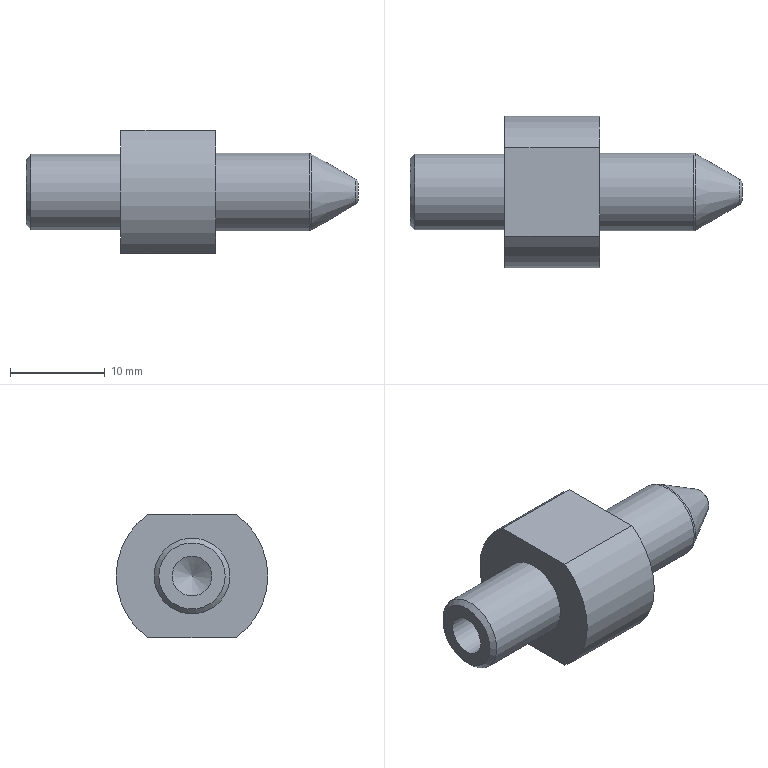Part | NX | features BREP 1 | 1 solid | 16 faces | box 35.023 x 16 x 13 mm | volume 2792 mm3 | plane 6 | cylinder 5 | cone 3 | torus 2 | commonest cylinder face diameters 16 x2 4.2 x1 8 x1 8.2 x1
STEP:
#1=CARTESIAN_POINT('',(2.489,-4.664,-6.5));
#2=VERTEX_POINT('',#1);
#3=CARTESIAN_POINT('',(2.489,-4.664,6.5));
#4=VERTEX_POINT('',#3);
#5=CARTESIAN_POINT('',(2.489,0.,0.));
#6=DIRECTION('',(-1.,0.,0.));
#7=DIRECTION('',(0.,-1.,0.));
#8=AXIS2_PLACEMENT_3D('',#5,#6,#7);
#9=CIRCLE('',#8,8.);
#10=EDGE_CURVE('',#2,#4,#9,.T.);
#11=ORIENTED_EDGE('',*,*,#10,.T.);
#12=CARTESIAN_POINT('',(-7.511,-4.664,6.5));
#13=VERTEX_POINT('',#12);
#14=CARTESIAN_POINT('',(-17.511,-4.664,6.5));
#15=DIRECTION('',(-1.,0.,0.));
#16=VECTOR('',#15,1000.);
#17=LINE('',#14,#16);
#18=EDGE_CURVE('',#4,#13,#17,.T.);
#19=ORIENTED_EDGE('',*,*,#18,.T.);
#20=CARTESIAN_POINT('',(-7.511,-4.664,-6.5));
#21=VERTEX_POINT('',#20);
#22=CARTESIAN_POINT('',(-7.511,0.,0.));
#23=DIRECTION('',(-1.,0.,0.));
#24=DIRECTION('',(0.,-1.,0.));
#25=AXIS2_PLACEMENT_3D('',#22,#23,#24);
#26=CIRCLE('',#25,8.);
#27=EDGE_CURVE('',#21,#13,#26,.T.);
#28=ORIENTED_EDGE('',*,*,#27,.F.);
#29=CARTESIAN_POINT('',(-17.511,-4.664,-6.5));
#30=DIRECTION('',(1.,0.,0.));
#31=VECTOR('',#30,1000.);
#32=LINE('',#29,#31);
#33=EDGE_CURVE('',#21,#2,#32,.T.);
#34=ORIENTED_EDGE('',*,*,#33,.T.);
#35=EDGE_LOOP('',(#11,#19,#28,#34));
#36=FACE_BOUND('',#35,.T.);
#37=CARTESIAN_POINT('',(-17.511,0.,0.));
#38=DIRECTION('',(-1.,0.,0.));
#39=DIRECTION('',(0.,1.,0.));
#40=AXIS2_PLACEMENT_3D('',#37,#38,#39);
#41=CYLINDRICAL_SURFACE('',#40,8.);
#42=ADVANCED_FACE('',(#36),#41,.T.);
#43=CARTESIAN_POINT('',(-17.511,3.5,0.));
#44=VERTEX_POINT('',#43);
#45=CARTESIAN_POINT('',(-17.511,0.,0.));
#46=DIRECTION('',(-1.,0.,0.));
#47=DIRECTION('',(0.,1.,0.));
#48=AXIS2_PLACEMENT_3D('',#45,#46,#47);
#49=CIRCLE('',#48,3.5);
#50=EDGE_CURVE('',#44,#44,#49,.T.);
#51=ORIENTED_EDGE('',*,*,#50,.T.);
#52=EDGE_LOOP('',(#51));
#53=FACE_BOUND('',#52,.T.);
#54=CARTESIAN_POINT('',(-17.511,0.,2.1));
#55=VERTEX_POINT('',#54);
#56=CARTESIAN_POINT('',(-17.511,0.,0.));
#57=DIRECTION('',(-1.,0.,0.));
#58=DIRECTION('',(0.,0.,1.));
#59=AXIS2_PLACEMENT_3D('',#56,#57,#58);
#60=CIRCLE('',#59,2.1);
#61=EDGE_CURVE('',#55,#55,#60,.T.);
#62=ORIENTED_EDGE('',*,*,#61,.F.);
#63=EDGE_LOOP('',(#62));
#64=FACE_BOUND('',#63,.T.);
#65=CARTESIAN_POINT('',(-17.511,4.,0.));
#66=DIRECTION('',(1.,0.,0.));
#67=DIRECTION('',(0.,-1.,0.));
#68=AXIS2_PLACEMENT_3D('',#65,#66,#67);
#69=PLANE('',#68);
#70=ADVANCED_FACE('',(#53,#64),#69,.F.);
#71=CARTESIAN_POINT('',(17.511,-0.9113,0.));
#72=VERTEX_POINT('',#71);
#73=CARTESIAN_POINT('',(17.511,0.,0.));
#74=DIRECTION('',(1.,0.,0.));
#75=DIRECTION('',(0.,-1.,0.));
#76=AXIS2_PLACEMENT_3D('',#73,#74,#75);
#77=CIRCLE('',#76,0.9113);
#78=EDGE_CURVE('',#72,#72,#77,.T.);
#79=ORIENTED_EDGE('',*,*,#78,.T.);
#80=EDGE_LOOP('',(#79));
#81=FACE_BOUND('',#80,.T.);
#82=CARTESIAN_POINT('',(17.511,0.,0.));
#83=DIRECTION('',(-1.,0.,0.));
#84=DIRECTION('',(0.,1.,0.));
#85=AXIS2_PLACEMENT_3D('',#82,#83,#84);
#86=PLANE('',#85);
#87=ADVANCED_FACE('',(#81),#86,.F.);
#88=CARTESIAN_POINT('',(17.261,1.344,0.));
#89=VERTEX_POINT('',#88);
#90=CARTESIAN_POINT('',(17.261,0.,0.));
#91=DIRECTION('',(-1.,0.,0.));
#92=DIRECTION('',(0.,1.,0.));
#93=AXIS2_PLACEMENT_3D('',#90,#91,#92);
#94=CIRCLE('',#93,1.344);
#95=EDGE_CURVE('',#89,#89,#94,.T.);
#96=ORIENTED_EDGE('',*,*,#95,.T.);
#97=EDGE_LOOP('',(#96));
#98=FACE_BOUND('',#97,.T.);
#99=CARTESIAN_POINT('',(12.605,4.033,0.));
#100=VERTEX_POINT('',#99);
#101=CARTESIAN_POINT('',(12.605,0.,0.));
#102=DIRECTION('',(1.,0.,0.));
#103=DIRECTION('',(0.,1.,0.));
#104=AXIS2_PLACEMENT_3D('',#101,#102,#103);
#105=CIRCLE('',#104,4.033);
#106=EDGE_CURVE('',#100,#100,#105,.T.);
#107=ORIENTED_EDGE('',*,*,#106,.T.);
#108=EDGE_LOOP('',(#107));
#109=FACE_BOUND('',#108,.T.);
#110=CARTESIAN_POINT('',(17.511,0.,0.));
#111=DIRECTION('',(-1.,0.,0.));
#112=DIRECTION('',(0.,1.,0.));
#113=AXIS2_PLACEMENT_3D('',#110,#111,#112);
#114=CONICAL_SURFACE('',#113,1.2,0.5236);
#115=ADVANCED_FACE('',(#98,#109),#114,.T.);
#116=CARTESIAN_POINT('',(12.355,4.1,0.));
#117=VERTEX_POINT('',#116);
#118=CARTESIAN_POINT('',(12.355,0.,0.));
#119=DIRECTION('',(-1.,0.,0.));
#120=DIRECTION('',(0.,1.,0.));
#121=AXIS2_PLACEMENT_3D('',#118,#119,#120);
#122=CIRCLE('',#121,4.1);
#123=EDGE_CURVE('',#117,#117,#122,.T.);
#124=ORIENTED_EDGE('',*,*,#123,.T.);
#125=EDGE_LOOP('',(#124));
#126=FACE_BOUND('',#125,.T.);
#127=CARTESIAN_POINT('',(2.489,-4.1,0.));
#128=VERTEX_POINT('',#127);
#129=CARTESIAN_POINT('',(2.489,0.,0.));
#130=DIRECTION('',(-1.,0.,0.));
#131=DIRECTION('',(0.,-1.,0.));
#132=AXIS2_PLACEMENT_3D('',#129,#130,#131);
#133=CIRCLE('',#132,4.1);
#134=EDGE_CURVE('',#128,#128,#133,.T.);
#135=ORIENTED_EDGE('',*,*,#134,.F.);
#136=EDGE_LOOP('',(#135));
#137=FACE_BOUND('',#136,.T.);
#138=CARTESIAN_POINT('',(-17.511,0.,0.));
#139=DIRECTION('',(-1.,0.,0.));
#140=DIRECTION('',(0.,1.,0.));
#141=AXIS2_PLACEMENT_3D('',#138,#139,#140);
#142=CYLINDRICAL_SURFACE('',#141,4.1);
#143=ADVANCED_FACE('',(#126,#137),#142,.T.);
#144=CARTESIAN_POINT('',(2.489,4.664,6.5));
#145=VERTEX_POINT('',#144);
#146=CARTESIAN_POINT('',(2.489,4.664,-6.5));
#147=VERTEX_POINT('',#146);
#148=CARTESIAN_POINT('',(2.489,0.,0.));
#149=DIRECTION('',(-1.,0.,0.));
#150=DIRECTION('',(0.,-1.,0.));
#151=AXIS2_PLACEMENT_3D('',#148,#149,#150);
#152=CIRCLE('',#151,8.);
#153=EDGE_CURVE('',#145,#147,#152,.T.);
#154=ORIENTED_EDGE('',*,*,#153,.F.);
#155=CARTESIAN_POINT('',(2.489,8.937,6.5));
#156=DIRECTION('',(0.,1.,0.));
#157=VECTOR('',#156,1000.);
#158=LINE('',#155,#157);
#159=EDGE_CURVE('',#4,#145,#158,.T.);
#160=ORIENTED_EDGE('',*,*,#159,.F.);
#161=ORIENTED_EDGE('',*,*,#10,.F.);
#162=CARTESIAN_POINT('',(2.489,7.21,-6.5));
#163=DIRECTION('',(0.,-1.,0.));
#164=VECTOR('',#163,1000.);
#165=LINE('',#162,#164);
#166=EDGE_CURVE('',#147,#2,#165,.T.);
#167=ORIENTED_EDGE('',*,*,#166,.F.);
#168=EDGE_LOOP('',(#154,#160,#161,#167));
#169=FACE_BOUND('',#168,.T.);
#170=ORIENTED_EDGE('',*,*,#134,.T.);
#171=EDGE_LOOP('',(#170));
#172=FACE_BOUND('',#171,.T.);
#173=CARTESIAN_POINT('',(2.489,4.1,0.));
#174=DIRECTION('',(-1.,0.,0.));
#175=DIRECTION('',(0.,1.,0.));
#176=AXIS2_PLACEMENT_3D('',#173,#174,#175);
#177=PLANE('',#176);
#178=ADVANCED_FACE('',(#169,#172),#177,.F.);
#179=CARTESIAN_POINT('',(-7.511,4.664,6.5));
#180=VERTEX_POINT('',#179);
#181=CARTESIAN_POINT('',(-7.511,4.664,-6.5));
#182=VERTEX_POINT('',#181);
#183=CARTESIAN_POINT('',(-7.511,0.,0.));
#184=DIRECTION('',(-1.,0.,0.));
#185=DIRECTION('',(0.,-1.,0.));
#186=AXIS2_PLACEMENT_3D('',#183,#184,#185);
#187=CIRCLE('',#186,8.);
#188=EDGE_CURVE('',#180,#182,#187,.T.);
#189=ORIENTED_EDGE('',*,*,#188,.F.);
#190=CARTESIAN_POINT('',(-17.511,4.664,6.5));
#191=DIRECTION('',(1.,0.,0.));
#192=VECTOR('',#191,1000.);
#193=LINE('',#190,#192);
#194=EDGE_CURVE('',#180,#145,#193,.T.);
#195=ORIENTED_EDGE('',*,*,#194,.T.);
#196=ORIENTED_EDGE('',*,*,#153,.T.);
#197=CARTESIAN_POINT('',(-17.511,4.664,-6.5));
#198=DIRECTION('',(-1.,0.,0.));
#199=VECTOR('',#198,1000.);
#200=LINE('',#197,#199);
#201=EDGE_CURVE('',#147,#182,#200,.T.);
#202=ORIENTED_EDGE('',*,*,#201,.T.);
#203=EDGE_LOOP('',(#189,#195,#196,#202));
#204=FACE_BOUND('',#203,.T.);
#205=CARTESIAN_POINT('',(-17.511,0.,0.));
#206=DIRECTION('',(-1.,0.,0.));
#207=DIRECTION('',(0.,1.,0.));
#208=AXIS2_PLACEMENT_3D('',#205,#206,#207);
#209=CYLINDRICAL_SURFACE('',#208,8.);
#210=ADVANCED_FACE('',(#204),#209,.T.);
#211=CARTESIAN_POINT('',(-7.511,-4.,0.));
#212=VERTEX_POINT('',#211);
#213=CARTESIAN_POINT('',(-7.511,0.,0.));
#214=DIRECTION('',(-1.,0.,0.));
#215=DIRECTION('',(0.,-1.,0.));
#216=AXIS2_PLACEMENT_3D('',#213,#214,#215);
#217=CIRCLE('',#216,4.);
#218=EDGE_CURVE('',#212,#212,#217,.T.);
#219=ORIENTED_EDGE('',*,*,#218,.F.);
#220=EDGE_LOOP('',(#219));
#221=FACE_BOUND('',#220,.T.);
#222=ORIENTED_EDGE('',*,*,#27,.T.);
#223=CARTESIAN_POINT('',(-7.511,8.,6.5));
#224=DIRECTION('',(0.,1.,0.));
#225=VECTOR('',#224,1000.);
#226=LINE('',#223,#225);
#227=EDGE_CURVE('',#13,#180,#226,.T.);
#228=ORIENTED_EDGE('',*,*,#227,.T.);
#229=ORIENTED_EDGE('',*,*,#188,.T.);
#230=CARTESIAN_POINT('',(-7.511,8.,-6.5));
#231=DIRECTION('',(0.,-1.,0.));
#232=VECTOR('',#231,1000.);
#233=LINE('',#230,#232);
#234=EDGE_CURVE('',#182,#21,#233,.T.);
#235=ORIENTED_EDGE('',*,*,#234,.T.);
#236=EDGE_LOOP('',(#222,#228,#229,#235));
#237=FACE_BOUND('',#236,.T.);
#238=CARTESIAN_POINT('',(-7.511,8.,0.));
#239=DIRECTION('',(1.,0.,0.));
#240=DIRECTION('',(0.,-1.,0.));
#241=AXIS2_PLACEMENT_3D('',#238,#239,#240);
#242=PLANE('',#241);
#243=ADVANCED_FACE('',(#221,#237),#242,.F.);
#244=CARTESIAN_POINT('',(-17.011,4.,0.));
#245=VERTEX_POINT('',#244);
#246=CARTESIAN_POINT('',(-17.011,0.,0.));
#247=DIRECTION('',(1.,0.,0.));
#248=DIRECTION('',(0.,1.,0.));
#249=AXIS2_PLACEMENT_3D('',#246,#247,#248);
#250=CIRCLE('',#249,4.);
#251=EDGE_CURVE('',#245,#245,#250,.T.);
#252=ORIENTED_EDGE('',*,*,#251,.T.);
#253=EDGE_LOOP('',(#252));
#254=FACE_BOUND('',#253,.T.);
#255=ORIENTED_EDGE('',*,*,#218,.T.);
#256=EDGE_LOOP('',(#255));
#257=FACE_BOUND('',#256,.T.);
#258=CARTESIAN_POINT('',(-17.511,0.,0.));
#259=DIRECTION('',(-1.,0.,0.));
#260=DIRECTION('',(0.,1.,0.));
#261=AXIS2_PLACEMENT_3D('',#258,#259,#260);
#262=CYLINDRICAL_SURFACE('',#261,4.);
#263=ADVANCED_FACE('',(#254,#257),#262,.T.);
#264=ORIENTED_EDGE('',*,*,#78,.F.);
#265=EDGE_LOOP('',(#264));
#266=FACE_BOUND('',#265,.T.);
#267=ORIENTED_EDGE('',*,*,#95,.F.);
#268=EDGE_LOOP('',(#267));
#269=FACE_BOUND('',#268,.T.);
#270=CARTESIAN_POINT('',(17.011,0.,0.));
#271=DIRECTION('',(-1.,0.,0.));
#272=DIRECTION('',(0.,1.,0.));
#273=AXIS2_PLACEMENT_3D('',#270,#271,#272);
#274=TOROIDAL_SURFACE('',#273,0.9113,0.5);
#275=ADVANCED_FACE('',(#266,#269),#274,.T.);
#276=ORIENTED_EDGE('',*,*,#106,.F.);
#277=EDGE_LOOP('',(#276));
#278=FACE_BOUND('',#277,.T.);
#279=ORIENTED_EDGE('',*,*,#123,.F.);
#280=EDGE_LOOP('',(#279));
#281=FACE_BOUND('',#280,.T.);
#282=CARTESIAN_POINT('',(12.355,0.,0.));
#283=DIRECTION('',(1.,0.,0.));
#284=DIRECTION('',(0.,-1.,0.));
#285=AXIS2_PLACEMENT_3D('',#282,#283,#284);
#286=TOROIDAL_SURFACE('',#285,3.6,0.5);
#287=ADVANCED_FACE('',(#278,#281),#286,.T.);
#288=CARTESIAN_POINT('',(-3.85,0.,0.));
#289=VERTEX_POINT('',#288);
#290=VERTEX_LOOP('',#289);
#291=FACE_BOUND('',#290,.T.);
#292=CARTESIAN_POINT('',(-5.111,0.,2.1));
#293=VERTEX_POINT('',#292);
#294=CARTESIAN_POINT('',(-5.111,0.,0.));
#295=DIRECTION('',(-1.,0.,0.));
#296=DIRECTION('',(0.,0.,1.));
#297=AXIS2_PLACEMENT_3D('',#294,#295,#296);
#298=CIRCLE('',#297,2.1);
#299=EDGE_CURVE('',#293,#293,#298,.T.);
#300=ORIENTED_EDGE('',*,*,#299,.T.);
#301=EDGE_LOOP('',(#300));
#302=FACE_BOUND('',#301,.T.);
#303=CARTESIAN_POINT('',(-5.111,0.,0.));
#304=DIRECTION('',(-1.,0.,0.));
#305=DIRECTION('',(0.,0.,-1.));
#306=AXIS2_PLACEMENT_3D('',#303,#304,#305);
#307=CONICAL_SURFACE('',#306,2.1,1.03);
#308=ADVANCED_FACE('',(#291,#302),#307,.F.);
#309=ORIENTED_EDGE('',*,*,#299,.F.);
#310=EDGE_LOOP('',(#309));
#311=FACE_BOUND('',#310,.T.);
#312=ORIENTED_EDGE('',*,*,#61,.T.);
#313=EDGE_LOOP('',(#312));
#314=FACE_BOUND('',#313,.T.);
#315=CARTESIAN_POINT('',(-17.511,0.,0.));
#316=DIRECTION('',(-1.,0.,0.));
#317=DIRECTION('',(0.,0.,-1.));
#318=AXIS2_PLACEMENT_3D('',#315,#316,#317);
#319=CYLINDRICAL_SURFACE('',#318,2.1);
#320=ADVANCED_FACE('',(#311,#314),#319,.F.);
#321=ORIENTED_EDGE('',*,*,#251,.F.);
#322=EDGE_LOOP('',(#321));
#323=FACE_BOUND('',#322,.T.);
#324=ORIENTED_EDGE('',*,*,#50,.F.);
#325=EDGE_LOOP('',(#324));
#326=FACE_BOUND('',#325,.T.);
#327=CARTESIAN_POINT('',(-17.511,0.,0.));
#328=DIRECTION('',(1.,0.,0.));
#329=DIRECTION('',(0.,-1.,0.));
#330=AXIS2_PLACEMENT_3D('',#327,#328,#329);
#331=CONICAL_SURFACE('',#330,3.5,0.7854);
#332=ADVANCED_FACE('',(#323,#326),#331,.T.);
#333=ORIENTED_EDGE('',*,*,#166,.T.);
#334=ORIENTED_EDGE('',*,*,#33,.F.);
#335=ORIENTED_EDGE('',*,*,#234,.F.);
#336=ORIENTED_EDGE('',*,*,#201,.F.);
#337=EDGE_LOOP('',(#333,#334,#335,#336));
#338=FACE_BOUND('',#337,.T.);
#339=CARTESIAN_POINT('',(-7.511,7.21,-6.5));
#340=DIRECTION('',(0.,0.,1.));
#341=DIRECTION('',(-1.,0.,0.));
#342=AXIS2_PLACEMENT_3D('',#339,#340,#341);
#343=PLANE('',#342);
#344=ADVANCED_FACE('',(#338),#343,.F.);
#345=ORIENTED_EDGE('',*,*,#159,.T.);
#346=ORIENTED_EDGE('',*,*,#194,.F.);
#347=ORIENTED_EDGE('',*,*,#227,.F.);
#348=ORIENTED_EDGE('',*,*,#18,.F.);
#349=EDGE_LOOP('',(#345,#346,#347,#348));
#350=FACE_BOUND('',#349,.T.);
#351=CARTESIAN_POINT('',(-7.511,8.937,6.5));
#352=DIRECTION('',(0.,0.,-1.));
#353=DIRECTION('',(1.,0.,0.));
#354=AXIS2_PLACEMENT_3D('',#351,#352,#353);
#355=PLANE('',#354);
#356=ADVANCED_FACE('',(#350),#355,.F.);
#357=CLOSED_SHELL('',(#42,#70,#87,#115,#143,#178,#210,#243,#263,#275,#287,#308,#320,#332,#344,#356));
#358=MANIFOLD_SOLID_BREP('',#357);
#359=(LENGTH_UNIT()NAMED_UNIT(*)SI_UNIT(.MILLI.,.METRE.));
#360=UNCERTAINTY_MEASURE_WITH_UNIT(LENGTH_MEASURE(0.00001),#359,'','');
#361=(NAMED_UNIT(*)PLANE_ANGLE_UNIT()SI_UNIT($,.RADIAN.));
#362=(NAMED_UNIT(*)SI_UNIT($,.STERADIAN.)SOLID_ANGLE_UNIT());
#363=(GEOMETRIC_REPRESENTATION_CONTEXT(3)GLOBAL_UNCERTAINTY_ASSIGNED_CONTEXT((#360))GLOBAL_UNIT_ASSIGNED_CONTEXT((#359,#361,#362))REPRESENTATION_CONTEXT('',''));
#364=ADVANCED_BREP_SHAPE_REPRESENTATION('',(#358),#363);